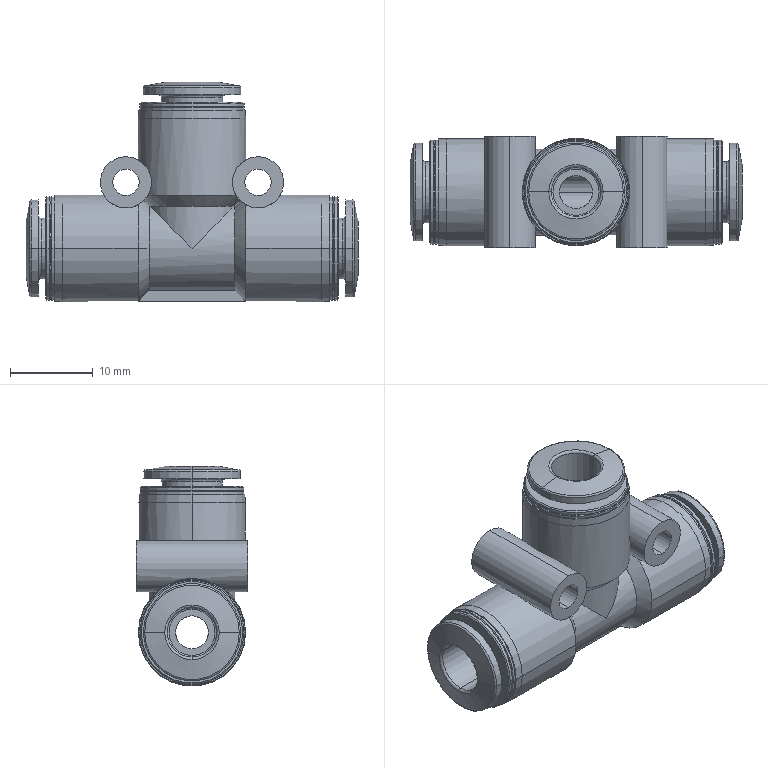Part | SolidWorks | features BaseBody 1 | 1 solid | 137 faces | box 40.2 x 13.5 x 26.6 mm | volume 5331 mm3 | cylinder 53 | cone 38 | torus 24 | plane 22 | commonest cylinder face diameters 12.6 x12 6 x6 7.4 x6 10.4 x6 11.8 x6 13 x5